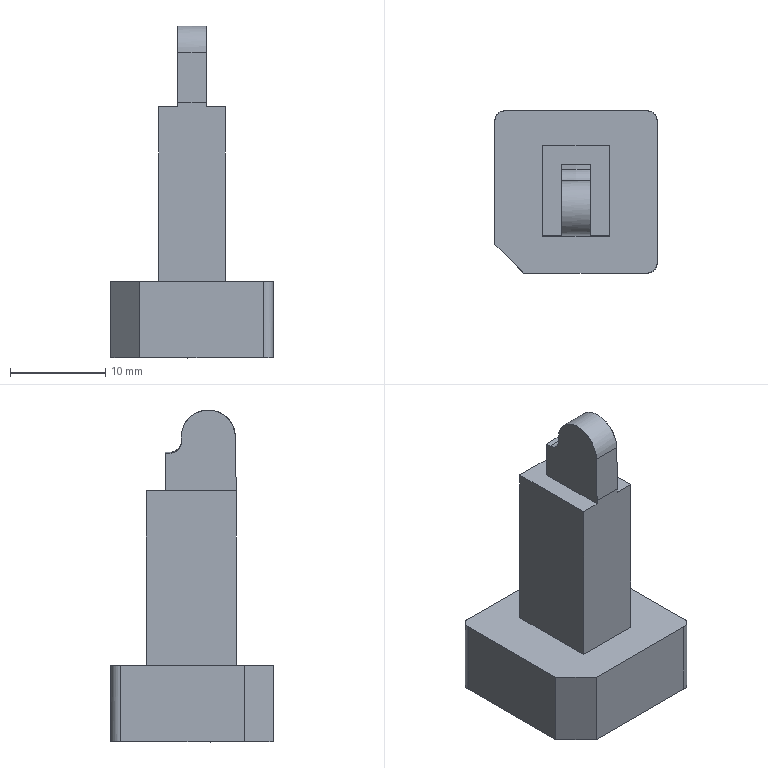NC program | PowerMill | posted with a generic post | part box 17 x 17 x 34.811 mm
Lines 1 to 1082 of 35253:
%
O0001
N104 ( POWERMILL CB  : 2026004.0)
N105 ( POST VER      : 2026.0.0.5161)
N106 ( OPTION FILE   : FANUC)
N107 ( OUTPUT WORKPLANE : WORLD)
N108 (  )
N109 ( TOOL LIST )
N110 (---------------------------------------)
N111 ( NO. | ID        | DIA.| TIP RAD|LENGTH)
N112 (---------------------------------------)
N113 (    1|D10C_1_1_1 |10.0 |  0.0   |90.28 )
N114 (    3|D10_1_1_1  |10.0 |  0.0   |89.96 )
N115 (    4|R1_1_1     | 2.0 |  1.0   |59.84 )
N116 (   14|D4_2_1     | 4.0 |  0.0   |63.64 )
N117 (   13|TEXT_D4_1_1| 4.0 |  0.3   |82.08 )
N118 (---------------------------------------)
N119 (  )
N120 ( NUMBER OF TOOLPATHS: 10.0 )
N121 ( ESTIMATED PROGRAM DURATION: 0 HOURS 6 MIN 1 SEC)
N122 (  )
N123 G00 G21 G80 G40 G17
N124 G90
N125 G54
N126 G53 Z0.0
N127 (---------------)
N128 ( START TOOLPATH : 粗公开粗01-扫面平行-D10C )
N129 (---------------)
N130 ( TOOL NO.    :1 )
N131 ( TOOL TYPE   : ENDMILL)
N132 ( TOOL ID     : D10C_1_1_1)
N133 ( TOOL DIA    : 10.0 LENGTH 90.28)
N134 T1
N135 M6
N136 S8000 M03
N137 G00 G90 X0.0 Y0.0
N138 G43 Z10.2 H1
N139
N140 G05 P10000 R4
N141 X16.15 Y11.15
N142 Z1.199
N143 G01 Z-0.001 F6000.0
N144 X11.15 F10000.0
N145 X-11.15
N146 Y5.575
N147 X11.15
N148 Y0.0
N149 X-11.15
N150 Y-5.575
N151 X11.15
N152 Y-11.15
N153 X-11.15
N154 X-16.15
N155 Z-0.202
N156 X-11.15
N157 X11.15
N158 Y-5.575
N159 X-11.15
N160 Y0.0
N161 X11.15
N162 Y5.575
N163 X-11.15
N164 Y11.15
N165 X11.15
N166 X16.15
N167 G00 Z10.2
N168 G05 P0
N169 (---------------)
N170 ( END TOOLPATH : 粗公开粗01-扫面平行-D10C )
N171 (---------------)
N172 ( START TOOLPATH : 粗公开粗01-外形偏置-D10C )
N173 (---------------)
N174 G00 X0.0 Y0.0915 Z9.801
N175 G05 P10000 R4
N176 X6.8255 Y-17.555
N177 Z0.5645
N178 G01 Z-0.6355 F6000.0
N179 Y-17.0275 F10000.0
N180 G03 X2.078 Y-12.28 I-4.7475 J0.0
N181 G01 X-10.156
N182 G02 X-11.156 Y-11.28 I0.0 J1.0
N183 G01 Y11.463
N184 G02 X-10.156 Y12.463 I1.0 J0.0
N185 G01 X10.156
N186 G02 X11.156 Y11.463 I0.0 J-1.0
N187 G01 Y-11.28
N188 G02 X10.156 Y-12.28 I-1.0 J0.0
N189 G01 X2.078
N190 X1.7402 Y-8.2544
N191 X1.5469 Y-8.2706
N192 X-1.5469
N193 X-2.3203 Y-8.2057
N194 X-3.0937 Y-8.0199
N195 X-3.8671 Y-7.6981
N196 X-4.6406 Y-7.2079
N197 X-5.0376 Y-6.8693
N198 X-5.414 Y-6.4752
N199 X-5.7108 Y-6.0959
N200 X-6.1625 Y-5.3225
N201 X-6.4542 Y-4.5491
N202 X-6.6142 Y-3.7756
N203 X-6.6566 Y-3.0022
N204 X-6.6408 Y0.0915
N205 X-6.5217 Y0.8649
N206 X-6.2762 Y1.6384
N207 X-6.1874 Y1.8463
N208 X-5.8829 Y2.4118
N209 X-5.414 Y3.0531
N210 X-4.6406 Y3.7854
N211 X-4.3982 Y3.9586
N212 X-3.8671 Y4.2756
N213 X-3.0937 Y4.5979
N214 X-2.3203 Y4.7837
N215 X-1.5469 Y4.8482
N216 X1.5469
N217 X2.3203 Y4.7837
N218 X3.0937 Y4.5979
N219 X3.8671 Y4.2756
N220 X4.3994 Y3.9586
N221 X4.6406 Y3.7854
N222 X5.2959 Y3.1852
N223 X5.8835 Y2.4118
N224 X6.2765 Y1.6384
N225 X6.5221 Y0.8649
N226 X6.6411 Y0.0915
N227 X6.6567 Y-3.0022
N228 X6.6143 Y-3.7756
N229 X6.4541 Y-4.5491
N230 X6.1874 Y-5.2685
N231 X5.7107 Y-6.0959
N232 X5.414 Y-6.4752
N233 X5.039 Y-6.8693
N234 X4.6406 Y-7.2079
N235 X3.968 Y-7.6428
N236 X3.0937 Y-8.0199
N237 X2.3203 Y-8.2057
N238 X1.7402 Y-8.2544
N239 X2.078 Y-12.28
N240 G00 Z3.2311
N241 G01 X6.8255 Y-17.555
N242 G00 Z0.1811
N243 G01 Z-1.0189 F6000.0
N244 Y-17.0275 F10000.0
N245 G03 X2.078 Y-12.28 I-4.7475 J0.0
N246 G01 X1.5469
N247 Y-8.7955
N248 X-1.5469
N249 X-2.3203 Y-8.7313
N250 X-3.0937 Y-8.5451
N251 X-3.4457 Y-8.4162
N252 X-3.8671 Y-8.2214
N253 X-4.6406 Y-7.7323
N254 X-5.414 Y-7.0008
N255 X-6.036 Y-6.0959
N256 X-6.1874 Y-5.7928
N257 X-6.3757 Y-5.3225
N258 X-6.5764 Y-4.5491
N259 X-6.6545 Y-3.7756
N260 X-6.6549 Y-3.0327
N261 X-6.6566 Y-3.0022
N262 X-6.6551 Y-2.7099
N263 X-6.6567 Y0.0915
N264 X-6.6158 Y0.8649
N265 X-6.4563 Y1.6384
N266 X-6.1874 Y2.3662
N267 X-5.7153 Y3.1852
N268 X-5.414 Y3.5734
N269 X-5.0466 Y3.9586
N270 X-4.6406 Y4.3052
N271 X-3.9846 Y4.7321
N272 X-3.0937 Y5.1178
N273 X-2.3203 Y5.3038
N274 X-1.5469 Y5.3683
N275 X1.5469
N276 X2.3203 Y5.3038
N277 X3.0937 Y5.1178
N278 X3.8671 Y4.7957
N279 X4.6406 Y4.3052
N280 X5.0461 Y3.9586
N281 X5.414 Y3.5734
N282 X5.7155 Y3.1852
N283 X6.1655 Y2.4118
N284 X6.4565 Y1.6384
N285 X6.6157 Y0.8649
N286 X6.6567 Y0.0915
N287 X6.6554 Y-2.7547
N288 X6.6567 Y-3.0022
N289 X6.6553 Y-3.0271
N290 X6.655 Y-3.7756
N291 X6.5769 Y-4.5491
N292 X6.3757 Y-5.3225
N293 X6.1874 Y-5.7928
N294 X6.0361 Y-6.0959
N295 X5.414 Y-7.0008
N296 X4.7534 Y-7.6428
N297 X3.8671 Y-8.2214
N298 X3.4454 Y-8.4162
N299 X3.0937 Y-8.5451
N300 X2.3203 Y-8.7313
N301 X1.5469 Y-8.7955
N302 Y-12.28
N303 X-10.156
N304 G02 X-11.156 Y-11.28 I0.0 J1.0
N305 G01 Y11.463
N306 G02 X-10.156 Y12.463 I1.0 J0.0
N307 G01 X10.156
N308 G02 X11.156 Y11.463 I0.0 J-1.0
N309 G01 Y-11.28
N310 G02 X10.156 Y-12.28 I-1.0 J0.0
N311 G01 X2.078
N312 G00 Z2.8476
N313 G01 X6.8255 Y-17.555
N314 G00 Z-0.2024
N315 G01 Z-1.4024 F6000.0
N316 Y-17.0275 F10000.0
N317 G03 X2.078 Y-12.28 I-4.7475 J0.0
N318 G01 X1.5469
N319 Y-9.1402
N320 X-1.5469
N321 X-2.3203 Y-9.0741
N322 X-3.0937 Y-8.8886
N323 X-3.8671 Y-8.5666
N324 X-4.1389 Y-8.4162
N325 X-4.6406 Y-8.0769
N326 X-5.1359 Y-7.6428
N327 X-5.414 Y-7.3439
N328 X-5.7769 Y-6.8693
N329 X-6.1874 Y-6.1372
N330 X-6.4803 Y-5.3225
N331 X-6.625 Y-4.5491
N332 X-6.6567 Y-3.7756
N333 X-6.6552 Y-3.0263
N334 X-6.6565 Y-3.0022
N335 X-6.655 Y-2.7099
N336 X-6.6566 Y0.0915
N337 X-6.6487 Y0.2419
N338 X-6.6474 Y0.8649
N339 X-6.5429 Y1.6384
N340 X-6.3128 Y2.4118
N341 X-6.1874 Y2.7107
N342 X-5.9382 Y3.1852
N343 X-5.414 Y3.9177
N344 X-4.6406 Y4.6492
N345 X-3.8671 Y5.1399
N346 X-3.0937 Y5.4621
N347 X-2.3203 Y5.648
N348 X-1.5469 Y5.7125
N349 X1.5469
N350 X2.3203 Y5.648
N351 X2.9529 Y5.5055
N352 X3.8671 Y5.1399
N353 X4.5283 Y4.7321
N354 X5.3772 Y3.9586
N355 X5.9386 Y3.1852
N356 X6.1874 Y2.7107
N357 X6.3133 Y2.4118
N358 X6.543 Y1.6384
N359 X6.6454 Y0.8649
N360 X6.6469 Y0.2756
N361 X6.6566 Y0.0915
N362 X6.6554 Y-2.7547
N363 X6.6566 Y-3.0022
N364 X6.6553 Y-3.0271
N365 X6.6552 Y-3.1398
N366 X6.6568 Y-3.7756
N367 X6.625 Y-4.5491
N368 X6.4796 Y-5.3225
N369 X6.2057 Y-6.0959
N370 X5.7766 Y-6.8693
N371 X5.414 Y-7.3439
N372 X5.1367 Y-7.6428
N373 X4.6406 Y-8.0769
N374 X4.1388 Y-8.4162
N375 X3.8671 Y-8.5666
N376 X3.0937 Y-8.8886
N377 X2.3203 Y-9.0741
N378 X1.5469 Y-9.1402
N379 Y-12.28
N380 X-10.156
N381 G02 X-11.156 Y-11.28 I0.0 J1.0
N382 G01 Y11.463
N383 G02 X-10.156 Y12.463 I1.0 J0.0
N384 G01 X10.156
N385 G02 X11.156 Y11.463 I0.0 J-1.0
N386 G01 Y-11.28
N387 G02 X10.156 Y-12.28 I-1.0 J0.0
N388 G01 X2.078
N389 G00 Z2.4642
N390 G01 X6.8255 Y-17.555
N391 G00 Z-0.5858
N392 G01 Z-1.7858 F6000.0
N393 Y-17.0275 F10000.0
N394 G03 X2.078 Y-12.28 I-4.7475 J0.0
N395 G01 X1.5469
N396 Y-9.376
N397 X-1.5469
N398 X-2.3203 Y-9.3122
N399 X-3.0937 Y-9.1262
N400 X-3.8671 Y-8.8041
N401 X-4.6406 Y-8.3135
N402 X-5.3611 Y-7.6428
N403 X-5.9261 Y-6.8693
N404 X-6.1874 Y-6.3741
N405 X-6.3045 Y-6.0959
N406 X-6.5375 Y-5.3225
N407 X-6.6464 Y-4.5491
N408 X-6.6473 Y-4.005
N409 X-6.6567 Y-3.7756
N410 X-6.6552 Y-3.0263
N411 X-6.6565 Y-3.0022
N412 X-6.655 Y-2.7099
N413 X-6.6566 Y0.0915
N414 X-6.6537 Y0.145
N415 X-6.6549 Y0.8649
N416 X-6.5879 Y1.6384
N417 X-6.3978 Y2.4118
N418 X-6.0709 Y3.1852
N419 X-5.5738 Y3.9586
N420 X-5.414 Y4.1549
N421 X-4.8315 Y4.7321
N422 X-4.6406 Y4.8867
N423 X-3.8671 Y5.3772
N424 X-3.5987 Y5.5055
N425 X-3.0937 Y5.6993
N426 X-2.3203 Y5.8852
N427 X-1.5469 Y5.9497
N428 X1.5469
N429 X2.3203 Y5.8852
N430 X3.0937 Y5.6993
N431 X3.8671 Y5.3772
N432 X4.6406 Y4.8867
N433 X4.8316 Y4.7321
N434 X5.414 Y4.1549
N435 X5.574 Y3.9586
N436 X6.0709 Y3.1852
N437 X6.3979 Y2.4118
N438 X6.5879 Y1.6384
N439 X6.6563 Y0.8649
N440 X6.6547 Y0.1263
N441 X6.6566 Y0.0915
N442 X6.6553 Y-2.7547
N443 X6.6566 Y-3.0022
N444 X6.6552 Y-3.0271
N445 Y-3.1398
N446 X6.6567 Y-3.7756
N447 X6.6457 Y-4.0441
N448 X6.6446 Y-4.5491
N449 X6.5371 Y-5.3225
N450 X6.3047 Y-6.0959
N451 X6.1874 Y-6.3741
N452 X5.9268 Y-6.8693
N453 X5.414 Y-7.5819
N454 X4.6406 Y-8.3135
N455 X3.8671 Y-8.8041
N456 X3.0937 Y-9.1262
N457 X2.8839 Y-9.1896
N458 X2.3203 Y-9.3122
N459 X1.5469 Y-9.376
N460 Y-12.28
N461 X-10.156
N462 G02 X-11.156 Y-11.28 I0.0 J1.0
N463 G01 Y11.463
N464 G02 X-10.156 Y12.463 I1.0 J0.0
N465 G01 X10.156
N466 G02 X11.156 Y11.463 I0.0 J-1.0
N467 G01 Y-11.28
N468 G02 X10.156 Y-12.28 I-1.0 J0.0
N469 G01 X2.078
N470 G00 Z2.0807
N471 G01 X6.8255 Y-17.555
N472 G00 Z-0.9693
N473 G01 Z-2.1693 F6000.0
N474 Y-17.0275 F10000.0
N475 G03 X2.078 Y-12.28 I-4.7475 J0.0
N476 G01 X1.5469
N477 Y-9.5373
N478 X-1.5469
N479 X-2.3203 Y-9.4726
N480 X-3.0937 Y-9.2866
N481 X-3.366 Y-9.1896
N482 X-3.8671 Y-8.9644
N483 X-4.6406 Y-8.4731
N484 X-5.414 Y-7.7416
N485 X-6.019 Y-6.8693
N486 X-6.1874 Y-6.5355
N487 X-6.3652 Y-6.0959
N488 X-6.5696 Y-5.3225
N489 X-6.6515 Y-4.5491
N490 X-6.6521 Y-3.8854
N491 X-6.6566 Y-3.7756
N492 X-6.6551 Y-3.0263
N493 X-6.6564 Y-3.0022
N494 X-6.6549 Y-2.7099
N495 X-6.6565 Y0.0915
N496 X-6.656 Y0.1016
N497 X-6.6567 Y0.8649
N498 X-6.6113 Y1.6384
N499 X-6.4474 Y2.4118
N500 X-6.1874 Y3.1089
N501 X-5.6947 Y3.9586
N502 X-5.414 Y4.3157
N503 X-5.0141 Y4.7321
N504 X-4.6406 Y5.0471
N505 X-3.9287 Y5.5055
N506 X-3.0937 Y5.8603
N507 X-2.3203 Y6.0462
N508 X-1.5469 Y6.1107
N509 X1.5469
N510 X2.3203 Y6.0462
N511 X3.0937 Y5.8603
N512 X3.8671 Y5.5381
N513 X4.6406 Y5.0471
N514 X5.0136 Y4.7321
N515 X5.414 Y4.3157
N516 X5.6943 Y3.9586
N517 X6.1521 Y3.1852
N518 X6.4478 Y2.4118
N519 X6.6109 Y1.6384
N520 X6.6567 Y0.8649
N521 X6.6564 Y0.0944
N522 X6.6565 Y0.0915
N523 X6.6553 Y-2.7547
N524 X6.6565 Y-3.0022
N525 X6.6552 Y-3.0271
N526 X6.6551 Y-3.1398
N527 X6.6567 Y-3.7756
N528 X6.6545 Y-3.8273
N529 X6.6542 Y-4.5491
N530 X6.5711 Y-5.3225
N531 X6.3638 Y-6.0959
N532 X6.1874 Y-6.5355
N533 X6.018 Y-6.8693
N534 X5.4972 Y-7.6428
N535 X4.7144 Y-8.4162
N536 X3.8671 Y-8.9644
N537 X3.3656 Y-9.1896
N538 X3.0937 Y-9.2866
N539 X2.3203 Y-9.4726
N540 X1.5469 Y-9.5373
N541 Y-12.28
N542 X-10.156
N543 G02 X-11.156 Y-11.28 I0.0 J1.0
N544 G01 Y11.463
N545 G02 X-10.156 Y12.463 I1.0 J0.0
N546 G01 X10.156
N547 G02 X11.156 Y11.463 I0.0 J-1.0
N548 G01 Y-11.28
N549 G02 X10.156 Y-12.28 I-1.0 J0.0
N550 G01 X2.078
N551 G00 Z1.6972
N552 G01 X6.8255 Y-17.555
N553 G00 Z-1.3528
N554 G01 Z-2.5528 F6000.0
N555 Y-17.0275 F10000.0
N556 G03 X2.078 Y-12.28 I-4.7475 J0.0
N557 G01 X1.5469
N558 Y-9.6361
N559 X-1.5469
N560 X-2.3203 Y-9.5719
N561 X-3.0937 Y-9.3855
N562 X-3.6043 Y-9.1896
N563 X-3.8671 Y-9.0638
N564 X-4.6406 Y-8.5746
N565 X-4.8358 Y-8.4162
N566 X-5.414 Y-7.8428
N567 X-5.5759 Y-7.6428
N568 X-6.0722 Y-6.8693
N569 X-6.3983 Y-6.0959
N570 X-6.5883 Y-5.3225
N571 X-6.656 Y-4.5491
N572 X-6.6561 Y-3.7867
N573 X-6.6566 Y-3.7756
N574 X-6.6562 Y-3.5642
N575 Y-3.0053
N576 X-6.6564 Y-3.0022
N577 X-6.6562 Y-2.9697
N578 X-6.6567 Y0.8649
N579 X-6.6242 Y1.6384
N580 X-6.4768 Y2.4118
N581 X-6.2004 Y3.1852
N582 X-5.7649 Y3.9586
N583 X-5.414 Y4.4188
N584 X-5.1208 Y4.7321
N585 X-4.6406 Y5.1498
N586 X-4.1153 Y5.5055
N587 X-3.8671 Y5.6418
N588 X-3.0937 Y5.9648
N589 X-2.3203 Y6.1506
N590 X-1.5469 Y6.2152
N591 X1.5469
N592 X2.3203 Y6.1506
N593 X3.0937 Y5.9648
N594 X3.8671 Y5.6418
N595 X4.1135 Y5.5055
N596 X4.6406 Y5.1498
N597 X5.1238 Y4.7321
N598 X5.414 Y4.4188
N599 X5.766 Y3.9586
N600 X6.1874 Y3.211
N601 X6.4757 Y2.4118
N602 X6.6236 Y1.6384
N603 X6.6567 Y0.8649
N604 X6.6563 Y-2.978
N605 X6.6565 Y-3.0022
N606 X6.6563 Y-3.0045
N607 Y-3.6426
N608 X6.6566 Y-3.7756
N609 X6.6563 Y-3.7839
N610 X6.6562 Y-4.5491
N611 X6.5883 Y-5.3225
N612 X6.3986 Y-6.0959
N613 X6.0721 Y-6.8693
N614 X5.5774 Y-7.6428
N615 X5.414 Y-7.8428
N616 X4.8372 Y-8.4162
N617 X4.6406 Y-8.5746
N618 X3.8671 Y-9.0638
N619 X3.6042 Y-9.1896
N620 X3.0937 Y-9.3855
N621 X2.3203 Y-9.5719
N622 X1.5469 Y-9.6361
N623 Y-12.28
N624 X-10.156
N625 G02 X-11.156 Y-11.28 I0.0 J1.0
N626 G01 Y11.463
N627 G02 X-10.156 Y12.463 I1.0 J0.0
N628 G01 X10.156
N629 G02 X11.156 Y11.463 I0.0 J-1.0
N630 G01 Y-11.28
N631 G02 X10.156 Y-12.28 I-1.0 J0.0
N632 G01 X2.078
N633 G00 Z1.3138
N634 G01 X6.8255 Y-17.555
N635 G00 Z-1.7362
N636 G01 Z-2.9362 F6000.0
N637 Y-17.0275 F10000.0
N638 G03 X2.078 Y-12.28 I-4.7475 J0.0
N639 G01 X1.5469
N640 Y-9.6808
N641 X-1.5469
N642 X-2.3203 Y-9.6148
N643 X-3.0937 Y-9.4292
N644 X-3.8671 Y-9.1067
N645 X-4.6406 Y-8.6177
N646 X-4.8872 Y-8.4162
N647 X-5.414 Y-7.8859
N648 X-5.6103 Y-7.6428
N649 X-6.092 Y-6.8693
N650 X-6.1874 Y-6.6789
N651 X-6.4132 Y-6.0959
N652 X-6.5954 Y-5.3225
N653 X-6.6566 Y-4.5491
N654 X-6.6567 Y0.8649
N655 X-6.6291 Y1.6384
N656 X-6.4877 Y2.4118
N657 X-6.2148 Y3.1852
N658 X-5.7946 Y3.9586
N659 X-5.414 Y4.4611
N660 X-5.1639 Y4.7321
N661 X-4.6406 Y5.1929
N662 X-4.184 Y5.5055
N663 X-3.8671 Y5.6833
N664 X-3.0937 Y6.0041
N665 X-2.3203 Y6.1914
N666 X-1.5469 Y6.2559
N667 X1.5469
N668 X2.3203 Y6.1914
N669 X3.0937 Y6.0041
N670 X3.8671 Y5.6833
N671 X4.184 Y5.5055
N672 X4.6406 Y5.1929
N673 X5.1637 Y4.7321
N674 X5.414 Y4.4611
N675 X5.7908 Y3.9586
N676 X6.1874 Y3.2541
N677 X6.4881 Y2.4118
N678 X6.6285 Y1.6384
N679 X6.6567 Y0.8649
N680 Y-4.5491
N681 X6.5956 Y-5.3225
N682 X6.4129 Y-6.0959
N683 X6.0928 Y-6.8693
N684 X5.6103 Y-7.6428
N685 X5.414 Y-7.8859
N686 X4.8862 Y-8.4162
N687 X4.6406 Y-8.6177
N688 X3.8671 Y-9.1067
N689 X3.7019 Y-9.1896
N690 X3.0937 Y-9.4292
N691 X2.3203 Y-9.6148
N692 X1.5469 Y-9.6808
N693 Y-12.28
N694 X-10.156
N695 G02 X-11.156 Y-11.28 I0.0 J1.0
N696 G01 Y11.463
N697 G02 X-10.156 Y12.463 I1.0 J0.0
N698 G01 X10.156
N699 G02 X11.156 Y11.463 I0.0 J-1.0
N700 G01 Y-11.28
N701 G02 X10.156 Y-12.28 I-1.0 J0.0
N702 G01 X2.078
N703 G00 Z0.9303
N704 G01 X6.8255 Y-17.555
N705 G00 Z-2.1197
N706 G01 Z-3.3197 F6000.0
N707 Y-17.0275 F10000.0
N708 G03 X2.078 Y-12.28 I-4.7475 J0.0
N709 G01 X1.5469
N710 Y-9.6926
N711 X-1.5469
N712 X-2.3203 Y-9.6296
N713 X-3.0937 Y-9.4437
N714 X-3.7298 Y-9.1896
N715 X-3.8604 Y-9.1094
N716 X-3.8671 Y-9.1066
N717 X-3.9406 Y-9.0602
N718 X-4.6406 Y-8.6303
N719 X-4.9015 Y-8.4162
N720 X-5.414 Y-7.898
N721 X-5.62 Y-7.6428
N722 X-6.102 Y-6.8693
N723 X-6.1459 Y-6.7617
N724 X-6.1874 Y-6.6789
N725 X-6.3332 Y-6.3024
N726 X-6.4174 Y-6.0959
N727 X-6.5974 Y-5.3225
N728 X-6.6566 Y-4.5491
N729 X-6.6567 Y0.8649
N730 X-6.6309 Y1.6384
N731 X-6.4949 Y2.4118
N732 X-6.2209 Y3.1852
N733 X-5.8052 Y3.9586
N734 X-5.414 Y4.4721
N735 X-5.1759 Y4.7321
N736 X-4.6406 Y5.2049
N737 X-4.1996 Y5.5055
N738 X-3.8671 Y5.6933
N739 X-3.0937 Y6.0124
N740 X-2.3203 Y6.2012
N741 X-1.5469 Y6.2651
N742 X1.5469 Y6.2677
N743 X2.3203 Y6.2012
N744 X3.0937 Y6.0124
N745 X3.8671 Y5.6933
N746 X4.201 Y5.5055
N747 X4.6406 Y5.2049
N748 X5.172 Y4.7321
N749 X5.414 Y4.4721
N750 X5.798 Y3.9586
N751 X6.1874 Y3.2643
N752 X6.4916 Y2.4118
N753 X6.63 Y1.6384
N754 X6.6568 Y0.8649
N755 X6.6567 Y-4.5491
N756 X6.5973 Y-5.3225
N757 X6.4173 Y-6.0959
N758 X6.102 Y-6.8693
N759 X5.6189 Y-7.6428
N760 X5.414 Y-7.898
N761 X4.9024 Y-8.4162
N762 X4.6406 Y-8.6303
N763 X3.9388 Y-9.0613
N764 X3.8671 Y-9.1066
N765 X3.8556 Y-9.1124
N766 X3.7299 Y-9.1896
N767 X3.0937 Y-9.4437
N768 X2.3203 Y-9.6296
N769 X1.5469 Y-9.6926
N770 Y-12.28
N771 X-10.156
N772 G02 X-11.156 Y-11.28 I0.0 J1.0
N773 G01 Y11.463
N774 G02 X-10.156 Y12.463 I1.0 J0.0
N775 G01 X10.156
N776 G02 X11.156 Y11.463 I0.0 J-1.0
N777 G01 Y-11.28
N778 G02 X10.156 Y-12.28 I-1.0 J0.0
N779 G01 X2.078
N780 G00 Z0.5468
N781 G01 X6.8255 Y-17.555
N782 G00 Z-2.5031
N783 G01 Z-3.7032 F6000.0
N784 Y-17.0275 F10000.0
N785 G03 X2.078 Y-12.28 I-4.7475 J0.0
N786 G01 X1.5469
N787 Y-9.7008
N788 X-1.5469
N789 X-2.3203 Y-9.6363
N790 X-3.0937 Y-9.4503
N791 X-3.7433 Y-9.1896
N792 X-4.6406 Y-8.6376
N793 X-4.91 Y-8.4162
N794 X-5.414 Y-7.9059
N795 X-5.6254 Y-7.6428
N796 X-6.1054 Y-6.8693
N797 X-6.1631 Y-6.7272
N798 X-6.1873 Y-6.6789
N799 X-6.281 Y-6.4371
N800 X-6.4195 Y-6.0959
N801 X-6.5986 Y-5.3225
N802 X-6.6567 Y-4.5491
N803 Y0.8649
N804 X-6.6325 Y1.6384
N805 X-6.501 Y2.4118
N806 X-6.2309 Y3.1852
N807 X-5.8134 Y3.9586
N808 X-5.414 Y4.4897
N809 X-5.192 Y4.7321
N810 X-4.6406 Y5.2215
N811 X-4.2303 Y5.5055
N812 X-3.8671 Y5.7119
N813 X-3.0937 Y6.0342
N814 X-2.3203 Y6.2201
N815 X-1.7478 Y6.2789
N816 X-0.7734 Y6.2977
N817 X1.5469 Y6.2858
N818 X2.3203 Y6.2201
N819 X3.0937 Y6.0342
N820 X3.8671 Y5.7119
N821 X4.2304 Y5.5055
N822 X4.6406 Y5.2215
N823 X5.192 Y4.7321
N824 X5.414 Y4.4897
N825 X5.8134 Y3.9586
N826 X6.1874 Y3.2827
N827 X6.4959 Y2.4118
N828 X6.6322 Y1.6384
N829 X6.6568 Y0.8649
N830 X6.6567 Y-4.5491
N831 X6.5986 Y-5.3225
N832 X6.4195 Y-6.0959
N833 X6.1054 Y-6.8693
N834 X5.6254 Y-7.6428
N835 X5.414 Y-7.9059
N836 X4.91 Y-8.4162
N837 X4.6406 Y-8.6376
N838 X3.7434 Y-9.1896
N839 X3.0937 Y-9.4503
N840 X2.3203 Y-9.6363
N841 X1.5469 Y-9.7008
N842 Y-12.28
N843 X-10.156
N844 G02 X-11.156 Y-11.28 I0.0 J1.0
N845 G01 Y11.463
N846 G02 X-10.156 Y12.463 I1.0 J0.0
N847 G01 X10.156
N848 G02 X11.156 Y11.463 I0.0 J-1.0
N849 G01 Y-11.28
N850 G02 X10.156 Y-12.28 I-1.0 J0.0
N851 G01 X2.078
N852 G00 Z0.1634
N853 G01 X6.8255 Y-17.555
N854 G00 Z-2.8866
N855 G01 Z-4.0866 F6000.0
N856 Y-17.0275 F10000.0
N857 G03 X2.078 Y-12.28 I-4.7475 J0.0
N858 G01 X1.5469
N859 Y-9.7075
N860 X-1.5469
N861 X-2.3203 Y-9.643
N862 X-3.0937 Y-9.457
N863 X-3.7568 Y-9.1896
N864 X-4.6406 Y-8.6444
N865 X-4.9176 Y-8.4162
N866 X-5.414 Y-7.9126
N867 X-5.6304 Y-7.6428
N868 X-6.1088 Y-6.8693
N869 X-6.1797 Y-6.694
N870 X-6.1873 Y-6.6789
N871 X-6.22 Y-6.5944
N872 X-6.4216 Y-6.0959
N873 X-6.5996 Y-5.3225
N874 X-6.6567 Y-4.5491
N875 X-6.6566 Y-4.5221
N876 X-6.6567 Y0.8649
N877 X-6.644 Y1.2697
N878 X-6.6432 Y1.6384
N879 X-6.5231 Y2.4118
N880 X-6.2771 Y3.1852
N881 X-5.8833 Y3.9586
N882 X-5.414 Y4.5995
N883 X-4.6406 Y5.3313
N884 X-4.3982 Y5.5055
N885 X-3.8671 Y5.8217
N886 X-3.0937 Y6.1448
N887 X-2.3203 Y6.3298
N888 X-0.7734 Y6.439
N889 X0.7734
N890 X2.3203 Y6.3298
N891 X3.0937 Y6.1448
N892 X3.8671 Y5.8217
N893 X4.3988 Y5.5055
N894 X4.6406 Y5.3313
N895 X5.2957 Y4.7321
N896 X5.8841 Y3.9586
N897 X6.2768 Y3.1852
N898 X6.5225 Y2.4118
N899 X6.6418 Y1.6384
N900 X6.6426 Y1.3096
N901 X6.6567 Y0.8649
N902 Y-4.5245
N903 X6.6568 Y-4.5491
N904 X6.5996 Y-5.3225
N905 X6.4216 Y-6.0959
N906 X6.1088 Y-6.8693
N907 X5.6304 Y-7.6428
N908 X5.414 Y-7.9126
N909 X4.9176 Y-8.4162
N910 X4.6406 Y-8.6444
N911 X3.7569 Y-9.1896
N912 X3.0937 Y-9.457
N913 X2.3203 Y-9.643
N914 X1.5469 Y-9.7075
N915 Y-12.28
N916 X-10.156
N917 G02 X-11.156 Y-11.28 I0.0 J1.0
N918 G01 Y11.463
N919 G02 X-10.156 Y12.463 I1.0 J0.0
N920 G01 X10.156
N921 G02 X11.156 Y11.463 I0.0 J-1.0
N922 G01 Y-11.28
N923 G02 X10.156 Y-12.28 I-1.0 J0.0
N924 G01 X2.078
N925 G00 Z-0.2201
N926 G01 X6.8255 Y-17.555
N927 G00 Z-3.2701
N928 G01 Z-4.4701 F6000.0
N929 Y-17.0275 F10000.0
N930 G03 X2.078 Y-12.28 I-4.7475 J0.0
N931 G01 X1.5469
N932 Y-9.7142
N933 X-1.5469
N934 X-2.3203 Y-9.6497
N935 X-3.0937 Y-9.4637
N936 X-3.7703 Y-9.1896
N937 X-4.6406 Y-8.6511
N938 X-4.9252 Y-8.4162
N939 X-5.414 Y-7.9193
N940 X-5.6354 Y-7.6428
N941 X-6.1121 Y-6.8693
N942 X-6.4237 Y-6.0959
N943 X-6.6006 Y-5.3225
N944 X-6.6567 Y-4.5491
N945 X-6.6566 Y-3.9517
N946 Y0.8649
N947 X-6.6557 Y0.8956
N948 X-6.6555 Y1.6384
N949 X-6.5812 Y2.4118
N950 X-6.3849 Y3.1852
N951 X-6.1874 Y3.684
N952 X-6.05 Y3.9586
N953 X-5.5434 Y4.7321
N954 X-5.414 Y4.8909
N955 X-4.7871 Y5.5055
N956 X-4.6406 Y5.623
N957 X-3.8671 Y6.1136
N958 X-3.5114 Y6.2789
N959 X-3.0937 Y6.4354
N960 X-2.3203 Y6.6228
N961 X-0.7734 Y6.7923
N962 X0.7734 Y6.7924
N963 X2.3203 Y6.6228
N964 X3.0937 Y6.4354
N965 X3.5116 Y6.2789
N966 X3.8671 Y6.1136
N967 X4.6406 Y5.623
N968 X4.7871 Y5.5055
N969 X5.414 Y4.8909
N970 X5.5432 Y4.7321
N971 X6.0502 Y3.9586
N972 X6.1874 Y3.684
N973 X6.3854 Y3.1852
N974 X6.5811 Y2.4118
N975 X6.6553 Y1.6384
N976 X6.6555 Y0.9026
N977 X6.6567 Y0.8649
N978 Y-4.0569
N979 X6.6568 Y-4.5491
N980 X6.6006 Y-5.3225
N981 X6.4237 Y-6.0959
N982 X6.1121 Y-6.8693
N983 X5.6354 Y-7.6428
N984 X5.414 Y-7.9193
N985 X4.9252 Y-8.4162
N986 X4.6406 Y-8.6511
N987 X3.7704 Y-9.1896
N988 X3.0937 Y-9.4637
N989 X2.3203 Y-9.6497
N990 X1.5469 Y-9.7142
N991 Y-12.28
N992 X-10.156
N993 G02 X-11.156 Y-11.28 I0.0 J1.0
N994 G01 Y11.463
N995 G02 X-10.156 Y12.463 I1.0 J0.0
N996 G01 X10.156
N997 G02 X11.156 Y11.463 I0.0 J-1.0
N998 G01 Y-11.28
N999 G02 X10.156 Y-12.28 I-1.0 J0.0
N1000 G01 X2.078
N1001 G00 Z-0.6035
N1002 G01 X6.8255 Y-17.555
N1003 G00 Z-3.6535
N1004 G01 Z-4.8535 F6000.0
N1005 Y-17.0275 F10000.0
N1006 G03 X2.078 Y-12.28 I-4.7475 J0.0
N1007 G01 X1.5469
N1008 Y-9.7209
N1009 X-1.5469
N1010 X-2.3203 Y-9.6564
N1011 X-3.0937 Y-9.4704
N1012 X-3.7838 Y-9.1896
N1013 X-4.6406 Y-8.6578
N1014 X-4.9327 Y-8.4162
N1015 X-5.414 Y-7.926
N1016 X-5.6404 Y-7.6428
N1017 X-6.1155 Y-6.8693
N1018 X-6.4258 Y-6.0959
N1019 X-6.6016 Y-5.3225
N1020 X-6.6567 Y-4.5491
N1021 Y2.4118
N1022 X-6.6435 Y3.1852
N1023 X-6.5284 Y3.9586
N1024 X-6.2871 Y4.7321
N1025 X-6.1874 Y4.9642
N1026 X-5.8988 Y5.5055
N1027 X-5.414 Y6.1712
N1028 X-4.6406 Y6.903
N1029 X-4.4355 Y7.0523
N1030 X-3.8671 Y7.3935
N1031 X-3.0937 Y7.7156
N1032 X-2.7015 Y7.8258
N1033 X-2.3203 Y7.9016
N1034 X-1.5469 Y7.966
N1035 X1.5469
N1036 X2.3203 Y7.9016
N1037 X2.7014 Y7.8258
N1038 X3.0937 Y7.7156
N1039 X3.8671 Y7.3935
N1040 X4.4355 Y7.0523
N1041 X4.6406 Y6.903
N1042 X5.3189 Y6.2789
N1043 X5.8988 Y5.5055
N1044 X6.1874 Y4.9642
N1045 X6.2871 Y4.7321
N1046 X6.5283 Y3.9586
N1047 X6.6435 Y3.1852
N1048 X6.6566 Y2.4118
N1049 X6.6568 Y-4.5491
N1050 X6.6016 Y-5.3225
N1051 X6.4258 Y-6.0959
N1052 X6.1874 Y-6.719
N1053 X6.1411 Y-6.7972
N1054 X6.1121 Y-6.8693
N1055 X5.7637 Y-7.4345
N1056 X5.6404 Y-7.6428
N1057 X5.414 Y-7.926
N1058 X4.9327 Y-8.4162
N1059 X4.6406 Y-8.6578
N1060 X3.7838 Y-9.1896
N1061 X3.0937 Y-9.4704
N1062 X2.3203 Y-9.6564
N1063 X1.5469 Y-9.7209
N1064 Y-12.28
N1065 X-10.156
N1066 G02 X-11.156 Y-11.28 I0.0 J1.0
N1067 G01 Y11.463
N1068 G02 X-10.156 Y12.463 I1.0 J0.0
N1069 G01 X10.156
N1070 G02 X11.156 Y11.463 I0.0 J-1.0
N1071 G01 Y-11.28
N1072 G02 X10.156 Y-12.28 I-1.0 J0.0
N1073 G01 X2.078
N1074 G00 Z-0.987
N1075 G01 X6.8255 Y-17.555
N1076 G00 Z-4.037
N1077 G01 Z-5.237 F6000.0
N1078 Y-17.0275 F10000.0
N1079 G03 X2.078 Y-12.28 I-4.7475 J0.0
N1080 G01 X1.5469
N1081 Y-9.7276
N1082 X-1.5469
N1083 X-2.3203 Y-9.6631
N1084 X-3.0937 Y-9.4771
N1085 X-3.7973 Y-9.1896
N1086 X-4.6406 Y-8.6645
N1087 X-4.9402 Y-8.4162
N1088 X-5.414 Y-7.9327
N1089 X-5.6453 Y-7.6428
N1090 X-6.1188 Y-6.8693
N1091 X-6.4279 Y-6.0959
N1092 X-6.6026 Y-5.3225
N1093 X-6.6567 Y-4.5491
N1094 Y2.4118
N1095 X-6.6435 Y3.1852
N1096 X-6.5284 Y3.9586
N1097 X-6.2871 Y4.7321
N1098 X-6.1874 Y4.9642
N1099 X-5.8989 Y5.5055
N1100 X-5.414 Y6.1712
N1101 X-4.6406 Y6.903
N1102 X-4.4356 Y7.0523
N1103 X-3.8671 Y7.3935
N1104 X-3.0937 Y7.7157
N1105 X-2.7015 Y7.8258
N1106 X-2.3203 Y7.9016
N1107 X-1.5469 Y7.966
N1108 X1.5469
N1109 X2.3203 Y7.9016
N1110 X2.7014 Y7.8258
N1111 X3.0937 Y7.7157
N1112 X3.8671 Y7.3935
N1113 X4.4355 Y7.0523
N1114 X4.6406 Y6.903
N1115 X5.3189 Y6.2789
N1116 X5.8989 Y5.5055
N1117 X6.1874 Y4.9642
N1118 X6.2871 Y4.7321
N1119 X6.5284 Y3.9586
N1120 X6.6435 Y3.1852
N1121 X6.6566 Y2.4118
N1122 X6.6568 Y-4.5491
N1123 X6.6026 Y-5.3225
N1124 X6.4279 Y-6.0959
N1125 X6.1874 Y-6.7257
N1126 X6.1323 Y-6.8189
N1127 X6.112 Y-6.8693
N1128 X5.8808 Y-7.2445
N1129 X5.6453 Y-7.6428
N1130 X5.414 Y-7.9327
N1131 X4.9402 Y-8.4162
N1132 X4.6406 Y-8.6645
N1133 X3.7973 Y-9.1896
N1134 X3.0937 Y-9.4771
N1135 X2.3203 Y-9.6631
N1136 X1.5469 Y-9.7276
N1137 Y-12.28
N1138 X-10.156
N1139 G02 X-11.156 Y-11.28 I0.0 J1.0
N1140 G01 Y11.463
N1141 G02 X-10.156 Y12.463 I1.0 J0.0
N1142 G01 X10.156
N1143 G02 X11.156 Y11.463 I0.0 J-1.0
N1144 G01 Y-11.28
N1145 G02 X10.156 Y-12.28 I-1.0 J0.0
N1146 G01 X2.078
N1147 G00 Z-1.3705
N1148 G01 X6.8255 Y-17.555
N1149 G00 Z-4.4205
N1150 G01 Z-5.6205 F6000.0
N1151 Y-17.0275 F10000.0
N1152 G03 X2.078 Y-12.28 I-4.7475 J0.0
N1153 G01 X1.5469
N1154 Y-9.7343
N1155 X-1.5469
N1156 X-2.3203 Y-9.6698
N1157 X-3.0937 Y-9.4838
N1158 X-3.8108 Y-9.1896
N1159 X-4.6406 Y-8.6712
N1160 X-4.9477 Y-8.4162
N1161 X-5.414 Y-7.9394
N1162 X-5.6503 Y-7.6428
N1163 X-6.1221 Y-6.8693
N1164 X-6.4299 Y-6.0959
N1165 X-6.6036 Y-5.3225
N1166 X-6.6567 Y-4.5491
N1167 Y2.4118
N1168 X-6.6435 Y3.1852
N1169 X-6.5284 Y3.9586
N1170 X-6.2871 Y4.7321
N1171 X-6.1874 Y4.9643
N1172 X-5.8989 Y5.5055
N1173 X-5.414 Y6.1712
N1174 X-4.6406 Y6.9031
N1175 X-4.4356 Y7.0523
N1176 X-3.8671 Y7.3935
N1177 X-3.0937 Y7.7157
N1178 X-2.7015 Y7.8258
N1179 X-2.3203 Y7.9016